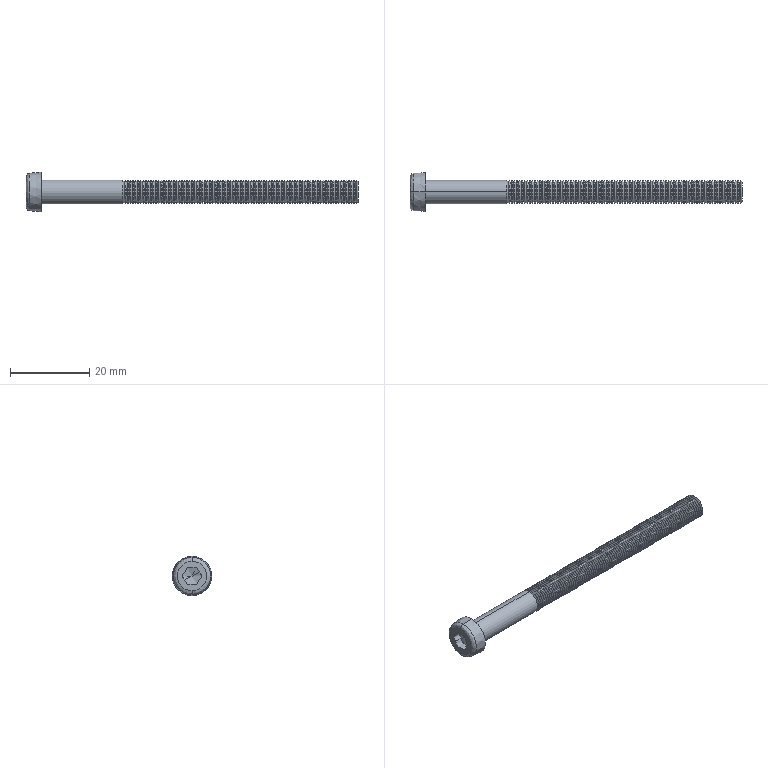Part | SolidWorks | features BaseBody 1, MoveFace 1 | 1 solid | 561 faces | box 83.9 x 10 x 10 mm | volume 2301 mm3 | cone 368 | cylinder 184 | spline 6 | plane 3 | commonest cylinder face diameters 6 x184